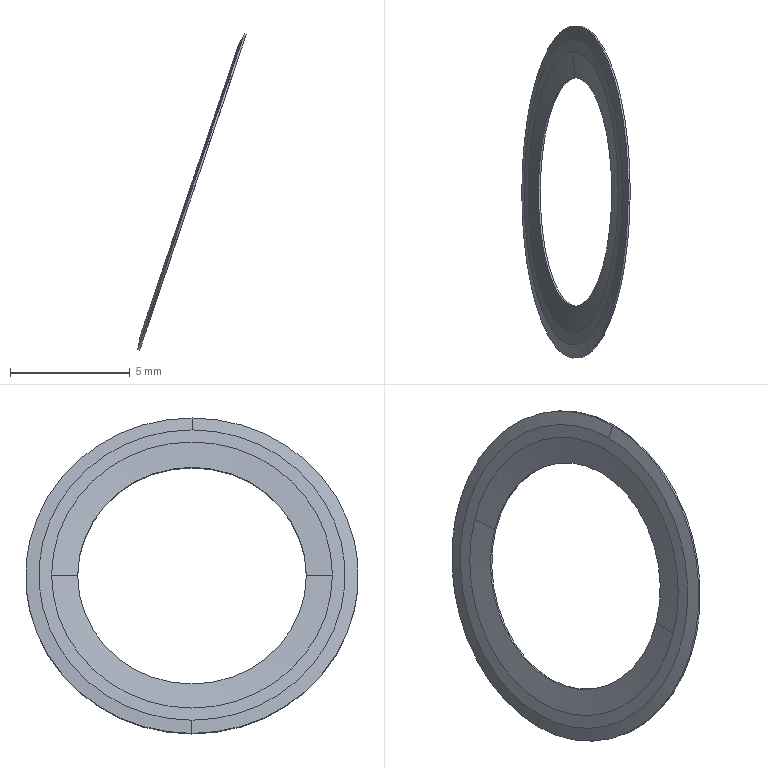Part | STEP file | 2026.6.15-Main Assembly图.sldasm-Part-225 | 1 solid | 14 faces | box 4.523 x 13.89 x 13.187 mm | volume 10.033 mm3 | cone 8 | cylinder 4 | plane 2 | commonest cylinder face diameters 9.54 x2 13.89 x2
STEP:
#1=CARTESIAN_POINT('',(-1660.905,1424.264,3253.413));
#2=VERTEX_POINT('',#1);
#3=CARTESIAN_POINT('',(-1660.649,1424.264,3253.911));
#4=VERTEX_POINT('',#3);
#5=CARTESIAN_POINT('',(-1660.649,1424.264,3253.911));
#6=DIRECTION('',(0.458,0.,0.8889));
#7=VECTOR('',#6,1000.);
#8=LINE('',#5,#7);
#9=EDGE_CURVE('',#2,#4,#8,.T.);
#10=ORIENTED_EDGE('',*,*,#9,.F.);
#11=CARTESIAN_POINT('',(-1664.995,1424.264,3241.302));
#12=VERTEX_POINT('',#11);
#13=CARTESIAN_POINT('',(-1662.95,1424.264,3247.357));
#14=DIRECTION('',(-0.9474,0.,0.3199));
#15=DIRECTION('',(-0.3199,0.,-0.9474));
#16=AXIS2_PLACEMENT_3D('',#13,#14,#15);
#17=CIRCLE('',#16,6.392);
#18=EDGE_CURVE('',#12,#2,#17,.T.);
#19=ORIENTED_EDGE('',*,*,#18,.F.);
#20=CARTESIAN_POINT('',(-1665.093,1424.264,3240.751));
#21=VERTEX_POINT('',#20);
#22=CARTESIAN_POINT('',(-1665.093,1424.264,3240.751));
#23=DIRECTION('',(-0.1747,0.,-0.9846));
#24=VECTOR('',#23,1000.);
#25=LINE('',#22,#24);
#26=EDGE_CURVE('',#12,#21,#25,.T.);
#27=ORIENTED_EDGE('',*,*,#26,.T.);
#28=CARTESIAN_POINT('',(-1662.871,1424.264,3247.331));
#29=DIRECTION('',(0.9474,0.,-0.3199));
#30=DIRECTION('',(-0.3199,0.,-0.9474));
#31=AXIS2_PLACEMENT_3D('',#28,#29,#30);
#32=CIRCLE('',#31,6.945);
#33=EDGE_CURVE('',#4,#21,#32,.T.);
#34=ORIENTED_EDGE('',*,*,#33,.F.);
#35=EDGE_LOOP('',(#10,#19,#27,#34));
#36=FACE_OUTER_BOUND('',#35,.T.);
#37=CARTESIAN_POINT('',(-1662.871,1424.264,3247.331));
#38=DIRECTION('',(0.9474,0.,-0.3199));
#39=DIRECTION('',(0.3199,0.,0.9474));
#40=AXIS2_PLACEMENT_3D('',#37,#38,#39);
#41=CONICAL_SURFACE('',#40,6.945,1.421);
#42=ADVANCED_FACE('',(#36),#41,.T.);
#43=CARTESIAN_POINT('',(-1660.57,1424.264,3253.884));
#44=VERTEX_POINT('',#43);
#45=CARTESIAN_POINT('',(-1650.384,1424.264,3250.444));
#46=DIRECTION('',(0.9474,0.,-0.3199));
#47=VECTOR('',#46,1000.);
#48=LINE('',#45,#47);
#49=EDGE_CURVE('',#4,#44,#48,.T.);
#50=ORIENTED_EDGE('',*,*,#49,.F.);
#51=ORIENTED_EDGE('',*,*,#33,.T.);
#52=CARTESIAN_POINT('',(-1665.014,1424.264,3240.724));
#53=VERTEX_POINT('',#52);
#54=CARTESIAN_POINT('',(-1654.828,1424.264,3237.284));
#55=DIRECTION('',(0.9474,0.,-0.3199));
#56=VECTOR('',#55,1000.);
#57=LINE('',#54,#56);
#58=EDGE_CURVE('',#21,#53,#57,.T.);
#59=ORIENTED_EDGE('',*,*,#58,.T.);
#60=CARTESIAN_POINT('',(-1662.792,1424.264,3247.304));
#61=DIRECTION('',(-0.9474,0.,0.3199));
#62=DIRECTION('',(-0.3199,0.,-0.9474));
#63=AXIS2_PLACEMENT_3D('',#60,#61,#62);
#64=CIRCLE('',#63,6.945);
#65=EDGE_CURVE('',#53,#44,#64,.T.);
#66=ORIENTED_EDGE('',*,*,#65,.T.);
#67=EDGE_LOOP('',(#50,#51,#59,#66));
#68=FACE_OUTER_BOUND('',#67,.T.);
#69=CARTESIAN_POINT('',(-1652.606,1424.264,3243.864));
#70=DIRECTION('',(0.9474,0.,-0.3199));
#71=DIRECTION('',(0.3199,0.,0.9474));
#72=AXIS2_PLACEMENT_3D('',#69,#70,#71);
#73=CYLINDRICAL_SURFACE('',#72,6.945);
#74=ADVANCED_FACE('',(#68),#73,.T.);
#75=ORIENTED_EDGE('',*,*,#18,.T.);
#76=CARTESIAN_POINT('',(-1662.95,1424.264,3247.357));
#77=DIRECTION('',(-0.9474,0.,0.3199));
#78=DIRECTION('',(-0.3199,0.,-0.9474));
#79=AXIS2_PLACEMENT_3D('',#76,#77,#78);
#80=CIRCLE('',#79,6.392);
#81=EDGE_CURVE('',#2,#12,#80,.T.);
#82=ORIENTED_EDGE('',*,*,#81,.T.);
#83=EDGE_LOOP('',(#75,#82));
#84=FACE_OUTER_BOUND('',#83,.T.);
#85=CARTESIAN_POINT('',(-1662.95,1418.407,3247.357));
#86=VERTEX_POINT('',#85);
#87=CARTESIAN_POINT('',(-1662.95,1430.122,3247.357));
#88=VERTEX_POINT('',#87);
#89=CARTESIAN_POINT('',(-1662.95,1424.264,3247.357));
#90=DIRECTION('',(0.9474,0.,-0.3199));
#91=DIRECTION('',(0.,-1.,0.));
#92=AXIS2_PLACEMENT_3D('',#89,#90,#91);
#93=CIRCLE('',#92,5.858);
#94=EDGE_CURVE('',#86,#88,#93,.T.);
#95=ORIENTED_EDGE('',*,*,#94,.T.);
#96=CARTESIAN_POINT('',(-1662.95,1424.264,3247.357));
#97=DIRECTION('',(0.9474,0.,-0.3199));
#98=DIRECTION('',(0.,-1.,0.));
#99=AXIS2_PLACEMENT_3D('',#96,#97,#98);
#100=CIRCLE('',#99,5.858);
#101=EDGE_CURVE('',#88,#86,#100,.T.);
#102=ORIENTED_EDGE('',*,*,#101,.T.);
#103=EDGE_LOOP('',(#95,#102));
#104=FACE_BOUND('',#103,.T.);
#105=CARTESIAN_POINT('',(-1662.95,1430.656,3247.357));
#106=DIRECTION('',(-0.9474,0.,0.3199));
#107=DIRECTION('',(0.,1.,0.));
#108=AXIS2_PLACEMENT_3D('',#105,#106,#107);
#109=PLANE('',#108);
#110=ADVANCED_FACE('',(#84,#104),#109,.T.);
#111=CARTESIAN_POINT('',(-1660.783,1424.264,3253.382));
#112=VERTEX_POINT('',#111);
#113=CARTESIAN_POINT('',(-1660.57,1424.264,3253.884));
#114=DIRECTION('',(0.3917,0.,0.9201));
#115=VECTOR('',#114,1000.);
#116=LINE('',#113,#115);
#117=EDGE_CURVE('',#112,#44,#116,.T.);
#118=ORIENTED_EDGE('',*,*,#117,.F.);
#119=CARTESIAN_POINT('',(-1662.831,1430.666,3247.317));
#120=VERTEX_POINT('',#119);
#121=CARTESIAN_POINT('',(-1662.831,1424.264,3247.317));
#122=DIRECTION('',(0.9474,0.,-0.3199));
#123=DIRECTION('',(0.3199,0.,0.9474));
#124=AXIS2_PLACEMENT_3D('',#121,#122,#123);
#125=CIRCLE('',#124,6.401);
#126=EDGE_CURVE('',#120,#112,#125,.T.);
#127=ORIENTED_EDGE('',*,*,#126,.F.);
#128=CARTESIAN_POINT('',(-1664.879,1424.264,3241.252));
#129=VERTEX_POINT('',#128);
#130=CARTESIAN_POINT('',(-1662.831,1424.264,3247.317));
#131=DIRECTION('',(0.9474,0.,-0.3199));
#132=DIRECTION('',(0.3199,0.,0.9474));
#133=AXIS2_PLACEMENT_3D('',#130,#131,#132);
#134=CIRCLE('',#133,6.401);
#135=EDGE_CURVE('',#129,#120,#134,.T.);
#136=ORIENTED_EDGE('',*,*,#135,.F.);
#137=CARTESIAN_POINT('',(-1665.014,1424.264,3240.724));
#138=DIRECTION('',(-0.2463,0.,-0.9692));
#139=VECTOR('',#138,1000.);
#140=LINE('',#137,#139);
#141=EDGE_CURVE('',#129,#53,#140,.T.);
#142=ORIENTED_EDGE('',*,*,#141,.T.);
#143=CARTESIAN_POINT('',(-1662.792,1424.264,3247.304));
#144=DIRECTION('',(-0.9474,0.,0.3199));
#145=DIRECTION('',(-0.3199,0.,-0.9474));
#146=AXIS2_PLACEMENT_3D('',#143,#144,#145);
#147=CIRCLE('',#146,6.945);
#148=EDGE_CURVE('',#44,#53,#147,.T.);
#149=ORIENTED_EDGE('',*,*,#148,.F.);
#150=EDGE_LOOP('',(#118,#127,#136,#142,#149));
#151=FACE_OUTER_BOUND('',#150,.T.);
#152=CARTESIAN_POINT('',(-1662.792,1424.264,3247.304));
#153=DIRECTION('',(0.9474,0.,-0.3199));
#154=DIRECTION('',(0.3199,0.,0.9474));
#155=AXIS2_PLACEMENT_3D('',#152,#153,#154);
#156=CONICAL_SURFACE('',#155,6.945,1.494);
#157=ADVANCED_FACE('',(#151),#156,.F.);
#158=CARTESIAN_POINT('',(-1662.871,1429.034,3247.331));
#159=VERTEX_POINT('',#158);
#160=CARTESIAN_POINT('',(-1662.95,1430.122,3247.357));
#161=DIRECTION('',(-0.0727,0.9971,0.02455));
#162=VECTOR('',#161,1000.);
#163=LINE('',#160,#162);
#164=EDGE_CURVE('',#159,#88,#163,.T.);
#165=ORIENTED_EDGE('',*,*,#164,.F.);
#166=CARTESIAN_POINT('',(-1661.345,1424.264,3251.85));
#167=VERTEX_POINT('',#166);
#168=CARTESIAN_POINT('',(-1662.871,1424.264,3247.331));
#169=DIRECTION('',(0.9474,0.,-0.3199));
#170=DIRECTION('',(-0.3199,0.,-0.9474));
#171=AXIS2_PLACEMENT_3D('',#168,#169,#170);
#172=CIRCLE('',#171,4.77);
#173=EDGE_CURVE('',#159,#167,#172,.T.);
#174=ORIENTED_EDGE('',*,*,#173,.T.);
#175=CARTESIAN_POINT('',(-1662.871,1419.494,3247.331));
#176=VERTEX_POINT('',#175);
#177=CARTESIAN_POINT('',(-1662.871,1424.264,3247.331));
#178=DIRECTION('',(0.9474,0.,-0.3199));
#179=DIRECTION('',(-0.3199,0.,-0.9474));
#180=AXIS2_PLACEMENT_3D('',#177,#178,#179);
#181=CIRCLE('',#180,4.77);
#182=EDGE_CURVE('',#167,#176,#181,.T.);
#183=ORIENTED_EDGE('',*,*,#182,.T.);
#184=CARTESIAN_POINT('',(-1662.95,1418.407,3247.357));
#185=DIRECTION('',(-0.0727,-0.9971,0.02455));
#186=VECTOR('',#185,1000.);
#187=LINE('',#184,#186);
#188=EDGE_CURVE('',#176,#86,#187,.T.);
#189=ORIENTED_EDGE('',*,*,#188,.T.);
#190=ORIENTED_EDGE('',*,*,#101,.F.);
#191=EDGE_LOOP('',(#165,#174,#183,#189,#190));
#192=FACE_OUTER_BOUND('',#191,.T.);
#193=CARTESIAN_POINT('',(-1662.95,1424.264,3247.357));
#194=DIRECTION('',(-0.9474,0.,0.3199));
#195=DIRECTION('',(0.,1.,0.));
#196=AXIS2_PLACEMENT_3D('',#193,#194,#195);
#197=CONICAL_SURFACE('',#196,5.858,1.494);
#198=ADVANCED_FACE('',(#192),#197,.F.);
#199=CARTESIAN_POINT('',(-1662.792,1430.122,3247.304));
#200=VERTEX_POINT('',#199);
#201=CARTESIAN_POINT('',(-1662.831,1430.666,3247.317));
#202=DIRECTION('',(-0.0727,0.9971,0.02455));
#203=VECTOR('',#202,1000.);
#204=LINE('',#201,#203);
#205=EDGE_CURVE('',#200,#120,#204,.T.);
#206=ORIENTED_EDGE('',*,*,#205,.F.);
#207=CARTESIAN_POINT('',(-1662.792,1418.407,3247.304));
#208=VERTEX_POINT('',#207);
#209=CARTESIAN_POINT('',(-1662.792,1424.264,3247.304));
#210=DIRECTION('',(0.9474,0.,-0.3199));
#211=DIRECTION('',(0.,-1.,0.));
#212=AXIS2_PLACEMENT_3D('',#209,#210,#211);
#213=CIRCLE('',#212,5.858);
#214=EDGE_CURVE('',#208,#200,#213,.T.);
#215=ORIENTED_EDGE('',*,*,#214,.F.);
#216=CARTESIAN_POINT('',(-1662.831,1417.863,3247.317));
#217=VERTEX_POINT('',#216);
#218=CARTESIAN_POINT('',(-1662.831,1417.863,3247.317));
#219=DIRECTION('',(-0.0727,-0.9971,0.02455));
#220=VECTOR('',#219,1000.);
#221=LINE('',#218,#220);
#222=EDGE_CURVE('',#208,#217,#221,.T.);
#223=ORIENTED_EDGE('',*,*,#222,.T.);
#224=CARTESIAN_POINT('',(-1662.831,1424.264,3247.317));
#225=DIRECTION('',(0.9474,0.,-0.3199));
#226=DIRECTION('',(0.3199,0.,0.9474));
#227=AXIS2_PLACEMENT_3D('',#224,#225,#226);
#228=CIRCLE('',#227,6.401);
#229=EDGE_CURVE('',#217,#129,#228,.T.);
#230=ORIENTED_EDGE('',*,*,#229,.T.);
#231=ORIENTED_EDGE('',*,*,#135,.T.);
#232=EDGE_LOOP('',(#206,#215,#223,#230,#231));
#233=FACE_OUTER_BOUND('',#232,.T.);
#234=CARTESIAN_POINT('',(-1662.831,1424.264,3247.317));
#235=DIRECTION('',(-0.9474,0.,0.3199));
#236=DIRECTION('',(0.,1.,0.));
#237=AXIS2_PLACEMENT_3D('',#234,#235,#236);
#238=CONICAL_SURFACE('',#237,6.401,1.494);
#239=ADVANCED_FACE('',(#233),#238,.T.);
#240=CARTESIAN_POINT('',(-1661.266,1424.264,3251.823));
#241=VERTEX_POINT('',#240);
#242=CARTESIAN_POINT('',(-1651.08,1424.264,3248.383));
#243=DIRECTION('',(0.9474,0.,-0.3199));
#244=VECTOR('',#243,1000.);
#245=LINE('',#242,#244);
#246=EDGE_CURVE('',#167,#241,#245,.T.);
#247=ORIENTED_EDGE('',*,*,#246,.F.);
#248=ORIENTED_EDGE('',*,*,#173,.F.);
#249=CARTESIAN_POINT('',(-1664.397,1424.264,3242.811));
#250=VERTEX_POINT('',#249);
#251=CARTESIAN_POINT('',(-1662.871,1424.264,3247.331));
#252=DIRECTION('',(0.9474,0.,-0.3199));
#253=DIRECTION('',(-0.3199,0.,-0.9474));
#254=AXIS2_PLACEMENT_3D('',#251,#252,#253);
#255=CIRCLE('',#254,4.77);
#256=EDGE_CURVE('',#250,#159,#255,.T.);
#257=ORIENTED_EDGE('',*,*,#256,.F.);
#258=CARTESIAN_POINT('',(-1664.318,1424.264,3242.785));
#259=VERTEX_POINT('',#258);
#260=CARTESIAN_POINT('',(-1654.132,1424.264,3239.345));
#261=DIRECTION('',(0.9474,0.,-0.3199));
#262=VECTOR('',#261,1000.);
#263=LINE('',#260,#262);
#264=EDGE_CURVE('',#250,#259,#263,.T.);
#265=ORIENTED_EDGE('',*,*,#264,.T.);
#266=CARTESIAN_POINT('',(-1662.792,1424.264,3247.304));
#267=DIRECTION('',(-0.9474,0.,0.3199));
#268=DIRECTION('',(-0.3199,0.,-0.9474));
#269=AXIS2_PLACEMENT_3D('',#266,#267,#268);
#270=CIRCLE('',#269,4.77);
#271=EDGE_CURVE('',#241,#259,#270,.T.);
#272=ORIENTED_EDGE('',*,*,#271,.F.);
#273=EDGE_LOOP('',(#247,#248,#257,#265,#272));
#274=FACE_OUTER_BOUND('',#273,.T.);
#275=CARTESIAN_POINT('',(-1652.606,1424.264,3243.864));
#276=DIRECTION('',(0.9474,0.,-0.3199));
#277=DIRECTION('',(0.3199,0.,0.9474));
#278=AXIS2_PLACEMENT_3D('',#275,#276,#277);
#279=CYLINDRICAL_SURFACE('',#278,4.77);
#280=ADVANCED_FACE('',(#274),#279,.F.);
#281=ORIENTED_EDGE('',*,*,#214,.T.);
#282=CARTESIAN_POINT('',(-1662.792,1424.264,3247.304));
#283=DIRECTION('',(0.9474,0.,-0.3199));
#284=DIRECTION('',(0.,-1.,0.));
#285=AXIS2_PLACEMENT_3D('',#282,#283,#284);
#286=CIRCLE('',#285,5.858);
#287=EDGE_CURVE('',#200,#208,#286,.T.);
#288=ORIENTED_EDGE('',*,*,#287,.T.);
#289=EDGE_LOOP('',(#281,#288));
#290=FACE_OUTER_BOUND('',#289,.T.);
#291=CARTESIAN_POINT('',(-1662.792,1424.264,3247.304));
#292=DIRECTION('',(-0.9474,0.,0.3199));
#293=DIRECTION('',(-0.3199,0.,-0.9474));
#294=AXIS2_PLACEMENT_3D('',#291,#292,#293);
#295=CIRCLE('',#294,4.77);
#296=EDGE_CURVE('',#259,#241,#295,.T.);
#297=ORIENTED_EDGE('',*,*,#296,.T.);
#298=ORIENTED_EDGE('',*,*,#271,.T.);
#299=EDGE_LOOP('',(#297,#298));
#300=FACE_BOUND('',#299,.T.);
#301=CARTESIAN_POINT('',(-1662.792,1429.034,3247.304));
#302=DIRECTION('',(0.9474,0.,-0.3199));
#303=DIRECTION('',(0.,-1.,0.));
#304=AXIS2_PLACEMENT_3D('',#301,#302,#303);
#305=PLANE('',#304);
#306=ADVANCED_FACE('',(#290,#300),#305,.T.);
#307=ORIENTED_EDGE('',*,*,#81,.F.);
#308=ORIENTED_EDGE('',*,*,#9,.T.);
#309=CARTESIAN_POINT('',(-1662.871,1424.264,3247.331));
#310=DIRECTION('',(0.9474,0.,-0.3199));
#311=DIRECTION('',(-0.3199,0.,-0.9474));
#312=AXIS2_PLACEMENT_3D('',#309,#310,#311);
#313=CIRCLE('',#312,6.945);
#314=EDGE_CURVE('',#21,#4,#313,.T.);
#315=ORIENTED_EDGE('',*,*,#314,.F.);
#316=ORIENTED_EDGE('',*,*,#26,.F.);
#317=EDGE_LOOP('',(#307,#308,#315,#316));
#318=FACE_OUTER_BOUND('',#317,.T.);
#319=CARTESIAN_POINT('',(-1662.871,1424.264,3247.331));
#320=DIRECTION('',(0.9474,0.,-0.3199));
#321=DIRECTION('',(0.3199,0.,0.9474));
#322=AXIS2_PLACEMENT_3D('',#319,#320,#321);
#323=CONICAL_SURFACE('',#322,6.945,1.421);
#324=ADVANCED_FACE('',(#318),#323,.T.);
#325=ORIENTED_EDGE('',*,*,#314,.T.);
#326=ORIENTED_EDGE('',*,*,#49,.T.);
#327=ORIENTED_EDGE('',*,*,#148,.T.);
#328=ORIENTED_EDGE('',*,*,#58,.F.);
#329=EDGE_LOOP('',(#325,#326,#327,#328));
#330=FACE_OUTER_BOUND('',#329,.T.);
#331=CARTESIAN_POINT('',(-1652.606,1424.264,3243.864));
#332=DIRECTION('',(0.9474,0.,-0.3199));
#333=DIRECTION('',(0.3199,0.,0.9474));
#334=AXIS2_PLACEMENT_3D('',#331,#332,#333);
#335=CYLINDRICAL_SURFACE('',#334,6.945);
#336=ADVANCED_FACE('',(#330),#335,.T.);
#337=CARTESIAN_POINT('',(-1662.831,1424.264,3247.317));
#338=DIRECTION('',(0.9474,0.,-0.3199));
#339=DIRECTION('',(0.3199,0.,0.9474));
#340=AXIS2_PLACEMENT_3D('',#337,#338,#339);
#341=CIRCLE('',#340,6.401);
#342=EDGE_CURVE('',#112,#217,#341,.T.);
#343=ORIENTED_EDGE('',*,*,#342,.F.);
#344=ORIENTED_EDGE('',*,*,#117,.T.);
#345=ORIENTED_EDGE('',*,*,#65,.F.);
#346=ORIENTED_EDGE('',*,*,#141,.F.);
#347=ORIENTED_EDGE('',*,*,#229,.F.);
#348=EDGE_LOOP('',(#343,#344,#345,#346,#347));
#349=FACE_OUTER_BOUND('',#348,.T.);
#350=CARTESIAN_POINT('',(-1662.792,1424.264,3247.304));
#351=DIRECTION('',(0.9474,0.,-0.3199));
#352=DIRECTION('',(0.3199,0.,0.9474));
#353=AXIS2_PLACEMENT_3D('',#350,#351,#352);
#354=CONICAL_SURFACE('',#353,6.945,1.494);
#355=ADVANCED_FACE('',(#349),#354,.F.);
#356=CARTESIAN_POINT('',(-1662.871,1424.264,3247.331));
#357=DIRECTION('',(0.9474,0.,-0.3199));
#358=DIRECTION('',(-0.3199,0.,-0.9474));
#359=AXIS2_PLACEMENT_3D('',#356,#357,#358);
#360=CIRCLE('',#359,4.77);
#361=EDGE_CURVE('',#176,#250,#360,.T.);
#362=ORIENTED_EDGE('',*,*,#361,.T.);
#363=ORIENTED_EDGE('',*,*,#256,.T.);
#364=ORIENTED_EDGE('',*,*,#164,.T.);
#365=ORIENTED_EDGE('',*,*,#94,.F.);
#366=ORIENTED_EDGE('',*,*,#188,.F.);
#367=EDGE_LOOP('',(#362,#363,#364,#365,#366));
#368=FACE_OUTER_BOUND('',#367,.T.);
#369=CARTESIAN_POINT('',(-1662.95,1424.264,3247.357));
#370=DIRECTION('',(-0.9474,0.,0.3199));
#371=DIRECTION('',(0.,1.,0.));
#372=AXIS2_PLACEMENT_3D('',#369,#370,#371);
#373=CONICAL_SURFACE('',#372,5.858,1.494);
#374=ADVANCED_FACE('',(#368),#373,.F.);
#375=ORIENTED_EDGE('',*,*,#287,.F.);
#376=ORIENTED_EDGE('',*,*,#205,.T.);
#377=ORIENTED_EDGE('',*,*,#126,.T.);
#378=ORIENTED_EDGE('',*,*,#342,.T.);
#379=ORIENTED_EDGE('',*,*,#222,.F.);
#380=EDGE_LOOP('',(#375,#376,#377,#378,#379));
#381=FACE_OUTER_BOUND('',#380,.T.);
#382=CARTESIAN_POINT('',(-1662.831,1424.264,3247.317));
#383=DIRECTION('',(-0.9474,0.,0.3199));
#384=DIRECTION('',(0.,1.,0.));
#385=AXIS2_PLACEMENT_3D('',#382,#383,#384);
#386=CONICAL_SURFACE('',#385,6.401,1.494);
#387=ADVANCED_FACE('',(#381),#386,.T.);
#388=ORIENTED_EDGE('',*,*,#182,.F.);
#389=ORIENTED_EDGE('',*,*,#246,.T.);
#390=ORIENTED_EDGE('',*,*,#296,.F.);
#391=ORIENTED_EDGE('',*,*,#264,.F.);
#392=ORIENTED_EDGE('',*,*,#361,.F.);
#393=EDGE_LOOP('',(#388,#389,#390,#391,#392));
#394=FACE_OUTER_BOUND('',#393,.T.);
#395=CARTESIAN_POINT('',(-1652.606,1424.264,3243.864));
#396=DIRECTION('',(0.9474,0.,-0.3199));
#397=DIRECTION('',(0.3199,0.,0.9474));
#398=AXIS2_PLACEMENT_3D('',#395,#396,#397);
#399=CYLINDRICAL_SURFACE('',#398,4.77);
#400=ADVANCED_FACE('',(#394),#399,.F.);
#401=CLOSED_SHELL('',(#42,#74,#110,#157,#198,#239,#280,#306,#324,#336,#355,#374,#387,#400));
#402=MANIFOLD_SOLID_BREP('',#401);
#403=CARTESIAN_POINT('',(0.,0.,0.));
#404=DIRECTION('',(0.,0.,1.));
#405=DIRECTION('',(1.,0.,0.));
#406=AXIS2_PLACEMENT_3D('',#403,#404,#405);
#407=(LENGTH_UNIT()NAMED_UNIT(*)SI_UNIT(.MILLI.,.METRE.));
#408=UNCERTAINTY_MEASURE_WITH_UNIT(LENGTH_MEASURE(0.00001),#407,'','');
#409=(NAMED_UNIT(*)PLANE_ANGLE_UNIT()SI_UNIT($,.RADIAN.));
#410=(NAMED_UNIT(*)SI_UNIT($,.STERADIAN.)SOLID_ANGLE_UNIT());
#411=(GEOMETRIC_REPRESENTATION_CONTEXT(3)GLOBAL_UNCERTAINTY_ASSIGNED_CONTEXT((#408))GLOBAL_UNIT_ASSIGNED_CONTEXT((#407,#409,#410))REPRESENTATION_CONTEXT('',''));
#412=ADVANCED_BREP_SHAPE_REPRESENTATION('',(#402,#406),#411);